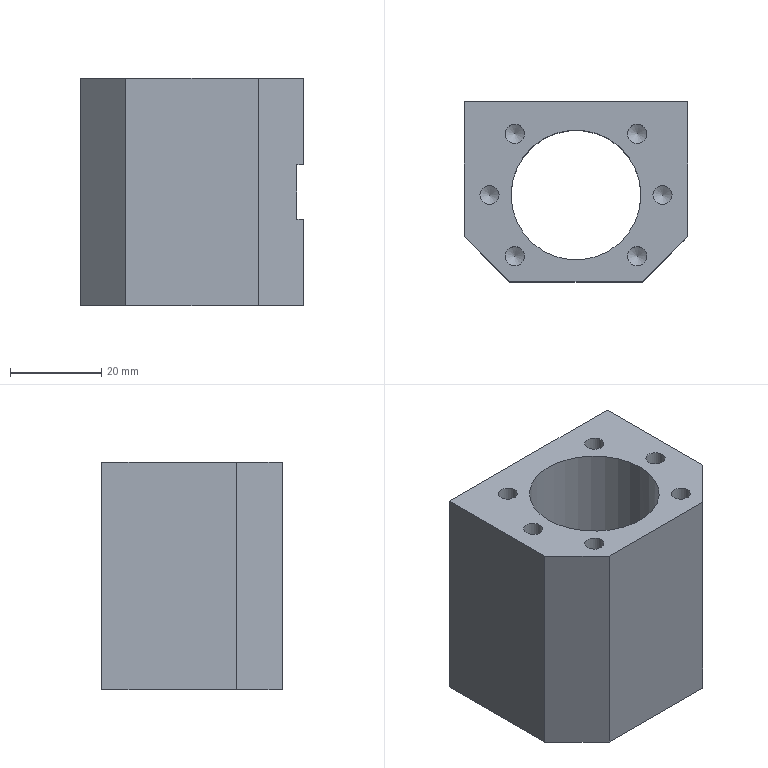Part | STEP file | 1 solid | 37 faces | box 49 x 39.6 x 50 mm | volume 57288 mm3 | cylinder 13 | plane 12 | cone 12 | commonest cylinder face diameters 4.2 x10 3.3 x2 28.5 x1